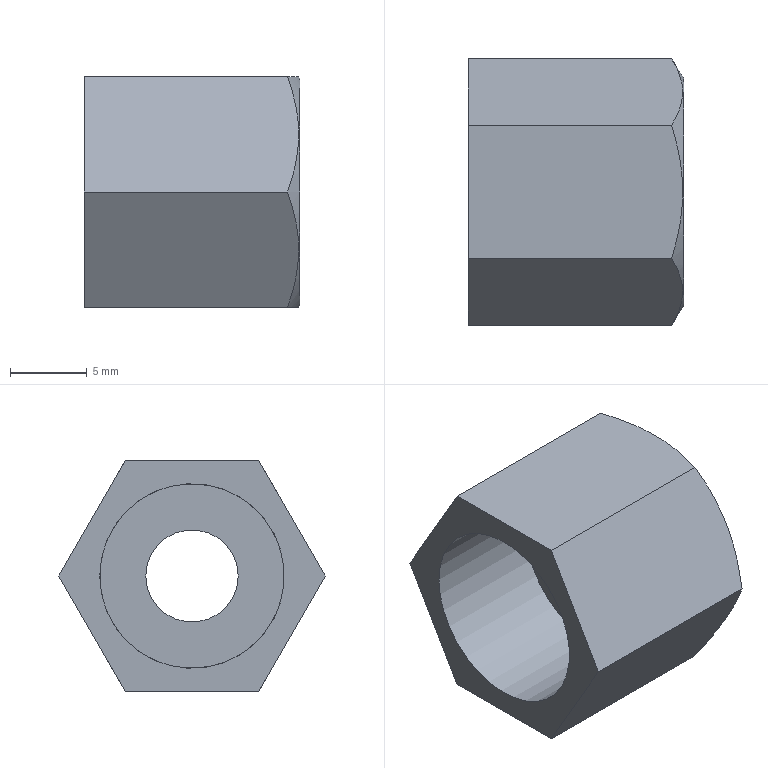Part | STEP file | 1-23.6 | 2 solids | 16 faces | box 14 x 17.321 x 15 mm | volume 1648 mm3 | plane 11 | cylinder 4 | cone 1 | commonest cylinder face diameters 6 x2 12 x2
STEP:
#1=CARTESIAN_POINT('',(0.,0.,0.));
#2=DIRECTION('',(0.,0.,1.));
#3=DIRECTION('',(1.,0.,0.));
#4=AXIS2_PLACEMENT_3D('',#1,#2,#3);
#5=CARTESIAN_POINT('',(0.,-4.33,7.5));
#6=VERTEX_POINT('',#5);
#7=CARTESIAN_POINT('',(0.,4.33,7.5));
#8=VERTEX_POINT('',#7);
#9=CARTESIAN_POINT('',(0.,-4.33,7.5));
#10=DIRECTION('',(0.,1.,0.));
#11=VECTOR('',#10,1.);
#12=LINE('',#9,#11);
#13=CARTESIAN_POINT('',(0.,0.,1.16));
#14=DIRECTION('',(-1.,0.,0.));
#15=DIRECTION('',(0.,0.,1.));
#16=AXIS2_PLACEMENT_3D('',#13,#14,#15);
#17=PLANE('',#16);
#18=CARTESIAN_POINT('',(6.34,-4.33));
#19=DIRECTION('',(0.,1.));
#20=VECTOR('',#19,1.);
#21=LINE('',#18,#20);
#22=(GEOMETRIC_REPRESENTATION_CONTEXT(2)PARAMETRIC_REPRESENTATION_CONTEXT()REPRESENTATION_CONTEXT('',''));
#23=DEFINITIONAL_REPRESENTATION('',(#21),#22);
#24=PCURVE('',#17,#23);
#25=CARTESIAN_POINT('',(7.,0.,7.5));
#26=DIRECTION('',(0.,0.,-1.));
#27=DIRECTION('',(0.,1.,0.));
#28=AXIS2_PLACEMENT_3D('',#25,#26,#27);
#29=PLANE('',#28);
#30=CARTESIAN_POINT('',(-4.33,-7.));
#31=DIRECTION('',(1.,0.));
#32=VECTOR('',#31,1.);
#33=LINE('',#30,#32);
#34=(GEOMETRIC_REPRESENTATION_CONTEXT(2)PARAMETRIC_REPRESENTATION_CONTEXT()REPRESENTATION_CONTEXT('',''));
#35=DEFINITIONAL_REPRESENTATION('',(#33),#34);
#36=PCURVE('',#29,#35);
#37=SURFACE_CURVE('',#12,(#24,#36),.PCURVE_S1.);
#38=EDGE_CURVE('',#6,#8,#37,.T.);
#39=ORIENTED_EDGE('',*,*,#38,.T.);
#40=CARTESIAN_POINT('',(0.,8.66,0.));
#41=VERTEX_POINT('',#40);
#42=CARTESIAN_POINT('',(0.,4.33,7.5));
#43=DIRECTION('',(0.,0.5,-0.866));
#44=VECTOR('',#43,1.);
#45=LINE('',#42,#44);
#46=CARTESIAN_POINT('',(6.34,4.33));
#47=DIRECTION('',(-0.866,0.5));
#48=VECTOR('',#47,1.);
#49=LINE('',#46,#48);
#50=(GEOMETRIC_REPRESENTATION_CONTEXT(2)PARAMETRIC_REPRESENTATION_CONTEXT()REPRESENTATION_CONTEXT('',''));
#51=DEFINITIONAL_REPRESENTATION('',(#49),#50);
#52=PCURVE('',#17,#51);
#53=CARTESIAN_POINT('',(7.,6.495,3.75));
#54=DIRECTION('',(0.,-0.866,-0.5));
#55=DIRECTION('',(0.,0.5,-0.866));
#56=AXIS2_PLACEMENT_3D('',#53,#54,#55);
#57=PLANE('',#56);
#58=CARTESIAN_POINT('',(-4.33,-7.));
#59=DIRECTION('',(1.,0.));
#60=VECTOR('',#59,1.);
#61=LINE('',#58,#60);
#62=(GEOMETRIC_REPRESENTATION_CONTEXT(2)PARAMETRIC_REPRESENTATION_CONTEXT()REPRESENTATION_CONTEXT('',''));
#63=DEFINITIONAL_REPRESENTATION('',(#61),#62);
#64=PCURVE('',#57,#63);
#65=SURFACE_CURVE('',#45,(#52,#64),.PCURVE_S1.);
#66=EDGE_CURVE('',#8,#41,#65,.T.);
#67=ORIENTED_EDGE('',*,*,#66,.T.);
#68=CARTESIAN_POINT('',(0.,4.33,-7.5));
#69=VERTEX_POINT('',#68);
#70=CARTESIAN_POINT('',(0.,8.66,0.));
#71=DIRECTION('',(0.,-0.5,-0.866));
#72=VECTOR('',#71,1.);
#73=LINE('',#70,#72);
#74=CARTESIAN_POINT('',(-1.16,8.66));
#75=DIRECTION('',(-0.866,-0.5));
#76=VECTOR('',#75,1.);
#77=LINE('',#74,#76);
#78=(GEOMETRIC_REPRESENTATION_CONTEXT(2)PARAMETRIC_REPRESENTATION_CONTEXT()REPRESENTATION_CONTEXT('',''));
#79=DEFINITIONAL_REPRESENTATION('',(#77),#78);
#80=PCURVE('',#17,#79);
#81=CARTESIAN_POINT('',(7.,6.495,-3.75));
#82=DIRECTION('',(0.,-0.866,0.5));
#83=DIRECTION('',(0.,-0.5,-0.866));
#84=AXIS2_PLACEMENT_3D('',#81,#82,#83);
#85=PLANE('',#84);
#86=CARTESIAN_POINT('',(-4.33,-7.));
#87=DIRECTION('',(1.,0.));
#88=VECTOR('',#87,1.);
#89=LINE('',#86,#88);
#90=(GEOMETRIC_REPRESENTATION_CONTEXT(2)PARAMETRIC_REPRESENTATION_CONTEXT()REPRESENTATION_CONTEXT('',''));
#91=DEFINITIONAL_REPRESENTATION('',(#89),#90);
#92=PCURVE('',#85,#91);
#93=SURFACE_CURVE('',#73,(#80,#92),.PCURVE_S1.);
#94=EDGE_CURVE('',#41,#69,#93,.T.);
#95=ORIENTED_EDGE('',*,*,#94,.T.);
#96=CARTESIAN_POINT('',(0.,-4.33,-7.5));
#97=VERTEX_POINT('',#96);
#98=CARTESIAN_POINT('',(0.,4.33,-7.5));
#99=DIRECTION('',(0.,-1.,0.));
#100=VECTOR('',#99,1.);
#101=LINE('',#98,#100);
#102=CARTESIAN_POINT('',(-8.66,4.33));
#103=DIRECTION('',(0.,-1.));
#104=VECTOR('',#103,1.);
#105=LINE('',#102,#104);
#106=(GEOMETRIC_REPRESENTATION_CONTEXT(2)PARAMETRIC_REPRESENTATION_CONTEXT()REPRESENTATION_CONTEXT('',''));
#107=DEFINITIONAL_REPRESENTATION('',(#105),#106);
#108=PCURVE('',#17,#107);
#109=CARTESIAN_POINT('',(7.,0.,-7.5));
#110=DIRECTION('',(0.,0.,1.));
#111=DIRECTION('',(0.,-1.,0.));
#112=AXIS2_PLACEMENT_3D('',#109,#110,#111);
#113=PLANE('',#112);
#114=CARTESIAN_POINT('',(-4.33,-7.));
#115=DIRECTION('',(1.,0.));
#116=VECTOR('',#115,1.);
#117=LINE('',#114,#116);
#118=(GEOMETRIC_REPRESENTATION_CONTEXT(2)PARAMETRIC_REPRESENTATION_CONTEXT()REPRESENTATION_CONTEXT('',''));
#119=DEFINITIONAL_REPRESENTATION('',(#117),#118);
#120=PCURVE('',#113,#119);
#121=SURFACE_CURVE('',#101,(#108,#120),.PCURVE_S1.);
#122=EDGE_CURVE('',#69,#97,#121,.T.);
#123=ORIENTED_EDGE('',*,*,#122,.T.);
#124=CARTESIAN_POINT('',(0.,-8.66,0.));
#125=VERTEX_POINT('',#124);
#126=CARTESIAN_POINT('',(0.,-4.33,-7.5));
#127=DIRECTION('',(0.,-0.5,0.866));
#128=VECTOR('',#127,1.);
#129=LINE('',#126,#128);
#130=CARTESIAN_POINT('',(-8.66,-4.33));
#131=DIRECTION('',(0.866,-0.5));
#132=VECTOR('',#131,1.);
#133=LINE('',#130,#132);
#134=(GEOMETRIC_REPRESENTATION_CONTEXT(2)PARAMETRIC_REPRESENTATION_CONTEXT()REPRESENTATION_CONTEXT('',''));
#135=DEFINITIONAL_REPRESENTATION('',(#133),#134);
#136=PCURVE('',#17,#135);
#137=CARTESIAN_POINT('',(7.,-6.495,-3.75));
#138=DIRECTION('',(0.,0.866,0.5));
#139=DIRECTION('',(0.,-0.5,0.866));
#140=AXIS2_PLACEMENT_3D('',#137,#138,#139);
#141=PLANE('',#140);
#142=CARTESIAN_POINT('',(-4.33,-7.));
#143=DIRECTION('',(1.,0.));
#144=VECTOR('',#143,1.);
#145=LINE('',#142,#144);
#146=(GEOMETRIC_REPRESENTATION_CONTEXT(2)PARAMETRIC_REPRESENTATION_CONTEXT()REPRESENTATION_CONTEXT('',''));
#147=DEFINITIONAL_REPRESENTATION('',(#145),#146);
#148=PCURVE('',#141,#147);
#149=SURFACE_CURVE('',#129,(#136,#148),.PCURVE_S1.);
#150=EDGE_CURVE('',#97,#125,#149,.T.);
#151=ORIENTED_EDGE('',*,*,#150,.T.);
#152=CARTESIAN_POINT('',(0.,-8.66,0.));
#153=DIRECTION('',(0.,0.5,0.866));
#154=VECTOR('',#153,1.);
#155=LINE('',#152,#154);
#156=CARTESIAN_POINT('',(-1.16,-8.66));
#157=DIRECTION('',(0.866,0.5));
#158=VECTOR('',#157,1.);
#159=LINE('',#156,#158);
#160=(GEOMETRIC_REPRESENTATION_CONTEXT(2)PARAMETRIC_REPRESENTATION_CONTEXT()REPRESENTATION_CONTEXT('',''));
#161=DEFINITIONAL_REPRESENTATION('',(#159),#160);
#162=PCURVE('',#17,#161);
#163=CARTESIAN_POINT('',(7.,-6.495,3.75));
#164=DIRECTION('',(0.,0.866,-0.5));
#165=DIRECTION('',(0.,0.5,0.866));
#166=AXIS2_PLACEMENT_3D('',#163,#164,#165);
#167=PLANE('',#166);
#168=CARTESIAN_POINT('',(-4.33,-7.));
#169=DIRECTION('',(1.,0.));
#170=VECTOR('',#169,1.);
#171=LINE('',#168,#170);
#172=(GEOMETRIC_REPRESENTATION_CONTEXT(2)PARAMETRIC_REPRESENTATION_CONTEXT()REPRESENTATION_CONTEXT('',''));
#173=DEFINITIONAL_REPRESENTATION('',(#171),#172);
#174=PCURVE('',#167,#173);
#175=SURFACE_CURVE('',#155,(#162,#174),.PCURVE_S1.);
#176=EDGE_CURVE('',#125,#6,#175,.T.);
#177=ORIENTED_EDGE('',*,*,#176,.T.);
#178=EDGE_LOOP('',(#39,#67,#95,#123,#151,#177));
#179=FACE_BOUND('',#178,.T.);
#180=CARTESIAN_POINT('',(0.,6.,0.));
#181=VERTEX_POINT('',#180);
#182=CARTESIAN_POINT('',(0.,0.,0.));
#183=DIRECTION('',(1.,0.,0.));
#184=DIRECTION('',(0.,1.,0.));
#185=AXIS2_PLACEMENT_3D('',#182,#183,#184);
#186=CIRCLE('',#185,6.);
#187=CARTESIAN_POINT('',(-1.16,6.));
#188=CARTESIAN_POINT('',(9.232,6.));
#189=CARTESIAN_POINT('',(4.036,-3.));
#190=CARTESIAN_POINT('',(-1.16,-12.));
#191=CARTESIAN_POINT('',(-6.356,-3.));
#192=CARTESIAN_POINT('',(-11.553,6.));
#193=CARTESIAN_POINT('',(-1.16,6.));
#194=(BOUNDED_CURVE()B_SPLINE_CURVE(2,(#187,#188,#189,#190,#191,#192,#193),.UNSPECIFIED.,.T.,.F.)B_SPLINE_CURVE_WITH_KNOTS((1,2,2,2,2,1),(-2.094,0.,2.094,4.189,6.283,8.378),.UNSPECIFIED.)CURVE()GEOMETRIC_REPRESENTATION_ITEM()RATIONAL_B_SPLINE_CURVE((1.,0.5,1.,0.5,1.,0.5,1.))REPRESENTATION_ITEM(''));
#195=(GEOMETRIC_REPRESENTATION_CONTEXT(2)PARAMETRIC_REPRESENTATION_CONTEXT()REPRESENTATION_CONTEXT('',''));
#196=DEFINITIONAL_REPRESENTATION('',(#194),#195);
#197=PCURVE('',#17,#196);
#198=CARTESIAN_POINT('',(0.,0.,0.));
#199=DIRECTION('',(1.,0.,0.));
#200=DIRECTION('',(0.,1.,0.));
#201=AXIS2_PLACEMENT_3D('',#198,#199,#200);
#202=CYLINDRICAL_SURFACE('',#201,6.);
#203=CARTESIAN_POINT('',(0.,0.));
#204=DIRECTION('',(1.,0.));
#205=VECTOR('',#204,1.);
#206=LINE('',#203,#205);
#207=(GEOMETRIC_REPRESENTATION_CONTEXT(2)PARAMETRIC_REPRESENTATION_CONTEXT()REPRESENTATION_CONTEXT('',''));
#208=DEFINITIONAL_REPRESENTATION('',(#206),#207);
#209=PCURVE('',#202,#208);
#210=SURFACE_CURVE('',#186,(#197,#209),.PCURVE_S1.);
#211=EDGE_CURVE('',#181,#181,#210,.T.);
#212=ORIENTED_EDGE('',*,*,#211,.T.);
#213=EDGE_LOOP('',(#212));
#214=FACE_BOUND('',#213,.T.);
#215=ADVANCED_FACE('',(#179,#214),#17,.T.);
#216=ORIENTED_EDGE('',*,*,#211,.T.);
#217=CARTESIAN_POINT('',(11.,6.,0.));
#218=VERTEX_POINT('',#217);
#219=CARTESIAN_POINT('',(0.,6.,0.));
#220=DIRECTION('',(1.,0.,0.));
#221=VECTOR('',#220,1.);
#222=LINE('',#219,#221);
#223=CARTESIAN_POINT('',(6.283,0.));
#224=DIRECTION('',(0.,1.));
#225=VECTOR('',#224,1.);
#226=LINE('',#223,#225);
#227=(GEOMETRIC_REPRESENTATION_CONTEXT(2)PARAMETRIC_REPRESENTATION_CONTEXT()REPRESENTATION_CONTEXT('',''));
#228=DEFINITIONAL_REPRESENTATION('',(#226),#227);
#229=PCURVE('',#202,#228);
#230=CARTESIAN_POINT('',(0.,0.));
#231=DIRECTION('',(0.,1.));
#232=VECTOR('',#231,1.);
#233=LINE('',#230,#232);
#234=(GEOMETRIC_REPRESENTATION_CONTEXT(2)PARAMETRIC_REPRESENTATION_CONTEXT()REPRESENTATION_CONTEXT('',''));
#235=DEFINITIONAL_REPRESENTATION('',(#233),#234);
#236=PCURVE('',#202,#235);
#237=SEAM_CURVE('',#222,(#229,#236),.PCURVE_S1.);
#238=EDGE_CURVE('',#181,#218,#237,.T.);
#239=ORIENTED_EDGE('',*,*,#238,.T.);
#240=CARTESIAN_POINT('',(11.,0.,0.));
#241=DIRECTION('',(1.,0.,0.));
#242=DIRECTION('',(0.,1.,0.));
#243=AXIS2_PLACEMENT_3D('',#240,#241,#242);
#244=CIRCLE('',#243,6.);
#245=CARTESIAN_POINT('',(0.,11.));
#246=DIRECTION('',(1.,0.));
#247=VECTOR('',#246,1.);
#248=LINE('',#245,#247);
#249=(GEOMETRIC_REPRESENTATION_CONTEXT(2)PARAMETRIC_REPRESENTATION_CONTEXT()REPRESENTATION_CONTEXT('',''));
#250=DEFINITIONAL_REPRESENTATION('',(#248),#249);
#251=PCURVE('',#202,#250);
#252=CARTESIAN_POINT('',(11.,-1.608,0.));
#253=DIRECTION('',(1.,0.,0.));
#254=DIRECTION('',(0.,0.,-1.));
#255=AXIS2_PLACEMENT_3D('',#252,#253,#254);
#256=PLANE('',#255);
#257=CARTESIAN_POINT('',(0.,1.608));
#258=DIRECTION('',(0.,1.));
#259=AXIS2_PLACEMENT_2D('',#257,#258);
#260=CIRCLE('',#259,6.);
#261=(GEOMETRIC_REPRESENTATION_CONTEXT(2)PARAMETRIC_REPRESENTATION_CONTEXT()REPRESENTATION_CONTEXT('',''));
#262=DEFINITIONAL_REPRESENTATION('',(#260),#261);
#263=PCURVE('',#256,#262);
#264=SURFACE_CURVE('',#244,(#251,#263),.PCURVE_S1.);
#265=EDGE_CURVE('',#218,#218,#264,.T.);
#266=ORIENTED_EDGE('',*,*,#265,.F.);
#267=ORIENTED_EDGE('',*,*,#238,.F.);
#268=EDGE_LOOP('',(#216,#239,#266,#267));
#269=FACE_BOUND('',#268,.F.);
#270=ADVANCED_FACE('',(#269),#202,.F.);
#271=ORIENTED_EDGE('',*,*,#38,.T.);
#272=CARTESIAN_POINT('',(13.213,4.33,7.5));
#273=VERTEX_POINT('',#272);
#274=CARTESIAN_POINT('',(0.,4.33,7.5));
#275=DIRECTION('',(1.,0.,0.));
#276=VECTOR('',#275,1.);
#277=LINE('',#274,#276);
#278=CARTESIAN_POINT('',(4.33,-7.));
#279=DIRECTION('',(0.,1.));
#280=VECTOR('',#279,1.);
#281=LINE('',#278,#280);
#282=(GEOMETRIC_REPRESENTATION_CONTEXT(2)PARAMETRIC_REPRESENTATION_CONTEXT()REPRESENTATION_CONTEXT('',''));
#283=DEFINITIONAL_REPRESENTATION('',(#281),#282);
#284=PCURVE('',#29,#283);
#285=CARTESIAN_POINT('',(-4.33,-7.));
#286=DIRECTION('',(0.,1.));
#287=VECTOR('',#286,1.);
#288=LINE('',#285,#287);
#289=(GEOMETRIC_REPRESENTATION_CONTEXT(2)PARAMETRIC_REPRESENTATION_CONTEXT()REPRESENTATION_CONTEXT('',''));
#290=DEFINITIONAL_REPRESENTATION('',(#288),#289);
#291=PCURVE('',#57,#290);
#292=SURFACE_CURVE('',#277,(#284,#291),.PCURVE_S1.);
#293=EDGE_CURVE('',#8,#273,#292,.T.);
#294=ORIENTED_EDGE('',*,*,#293,.T.);
#295=CARTESIAN_POINT('',(13.936,0.,7.5));
#296=VERTEX_POINT('',#295);
#297=CARTESIAN_POINT('',(13.213,4.33,7.5));
#298=CARTESIAN_POINT('',(13.936,2.01,7.5));
#299=CARTESIAN_POINT('',(13.936,0.,7.5));
#300=(BOUNDED_CURVE()B_SPLINE_CURVE(2,(#297,#298,#299),.UNSPECIFIED.,.F.,.F.)B_SPLINE_CURVE_WITH_KNOTS((3,3),(0.,1.),.PIECEWISE_BEZIER_KNOTS.)CURVE()GEOMETRIC_REPRESENTATION_ITEM()RATIONAL_B_SPLINE_CURVE((1.788,1.926,1.926))REPRESENTATION_ITEM(''));
#301=CARTESIAN_POINT('',(4.33,6.213));
#302=CARTESIAN_POINT('',(2.01,6.936));
#303=CARTESIAN_POINT('',(0.,6.936));
#304=(BOUNDED_CURVE()B_SPLINE_CURVE(2,(#301,#302,#303),.UNSPECIFIED.,.F.,.F.)B_SPLINE_CURVE_WITH_KNOTS((3,3),(0.,1.),.PIECEWISE_BEZIER_KNOTS.)CURVE()GEOMETRIC_REPRESENTATION_ITEM()RATIONAL_B_SPLINE_CURVE((1.788,1.926,1.926))REPRESENTATION_ITEM(''));
#305=(GEOMETRIC_REPRESENTATION_CONTEXT(2)PARAMETRIC_REPRESENTATION_CONTEXT()REPRESENTATION_CONTEXT('',''));
#306=DEFINITIONAL_REPRESENTATION('',(#304),#305);
#307=PCURVE('',#29,#306);
#308=CARTESIAN_POINT('',(14.,0.,0.));
#309=DIRECTION('',(-1.,0.,0.));
#310=DIRECTION('',(0.,0.,1.));
#311=AXIS2_PLACEMENT_3D('',#308,#309,#310);
#312=CONICAL_SURFACE('',#311,7.397,1.014);
#313=CARTESIAN_POINT('',(0.5236,0.7867));
#314=CARTESIAN_POINT('',(0.516,0.7631));
#315=CARTESIAN_POINT('',(0.5008,0.7174));
#316=CARTESIAN_POINT('',(0.4779,0.6528));
#317=CARTESIAN_POINT('',(0.4548,0.5921));
#318=CARTESIAN_POINT('',(0.4317,0.5352));
#319=CARTESIAN_POINT('',(0.4084,0.482));
#320=CARTESIAN_POINT('',(0.3849,0.4324));
#321=CARTESIAN_POINT('',(0.3614,0.3862));
#322=CARTESIAN_POINT('',(0.3378,0.3434));
#323=CARTESIAN_POINT('',(0.3141,0.3039));
#324=CARTESIAN_POINT('',(0.2903,0.2677));
#325=CARTESIAN_POINT('',(0.2664,0.2345));
#326=CARTESIAN_POINT('',(0.2424,0.2044));
#327=CARTESIAN_POINT('',(0.2184,0.1774));
#328=CARTESIAN_POINT('',(0.1943,0.1534));
#329=CARTESIAN_POINT('',(0.1701,0.1322));
#330=CARTESIAN_POINT('',(0.1459,0.114));
#331=CARTESIAN_POINT('',(0.1217,0.09862));
#332=CARTESIAN_POINT('',(0.09736,0.08608));
#333=CARTESIAN_POINT('',(0.07305,0.07635));
#334=CARTESIAN_POINT('',(0.04871,0.06941));
#335=CARTESIAN_POINT('',(0.02436,0.06525));
#336=CARTESIAN_POINT('',(0.00812,0.06433));
#337=CARTESIAN_POINT('',(0.,0.06433));
#338=B_SPLINE_CURVE_WITH_KNOTS('',3,(#313,#314,#315,#316,#317,#318,#319,#320,#321,#322,#323,#324,#325,#326,#327,#328,#329,#330,#331,#332,#333,#334,#335,#336,#337),.UNSPECIFIED.,.F.,.F.,(4,1,1,1,1,1,1,1,1,1,1,1,1,1,1,1,1,1,1,1,1,1,4),(0.,0.04545,0.09091,0.1364,0.1818,0.2273,0.2727,0.3182,0.3636,0.4091,0.4545,0.5,0.5455,0.5909,0.6364,0.6818,0.7273,0.7727,0.8182,0.8636,0.9091,0.9545,1.),.QUASI_UNIFORM_KNOTS.);
#339=(GEOMETRIC_REPRESENTATION_CONTEXT(2)PARAMETRIC_REPRESENTATION_CONTEXT()REPRESENTATION_CONTEXT('',''));
#340=DEFINITIONAL_REPRESENTATION('',(#338),#339);
#341=PCURVE('',#312,#340);
#342=SURFACE_CURVE('',#300,(#307,#341),.PCURVE_S1.);
#343=EDGE_CURVE('',#273,#296,#342,.T.);
#344=ORIENTED_EDGE('',*,*,#343,.T.);
#345=CARTESIAN_POINT('',(13.213,-4.33,7.5));
#346=VERTEX_POINT('',#345);
#347=CARTESIAN_POINT('',(13.936,0.,7.5));
#348=CARTESIAN_POINT('',(13.936,-2.01,7.5));
#349=CARTESIAN_POINT('',(13.213,-4.33,7.5));
#350=(BOUNDED_CURVE()B_SPLINE_CURVE(2,(#347,#348,#349),.UNSPECIFIED.,.F.,.F.)B_SPLINE_CURVE_WITH_KNOTS((3,3),(0.,1.),.PIECEWISE_BEZIER_KNOTS.)CURVE()GEOMETRIC_REPRESENTATION_ITEM()RATIONAL_B_SPLINE_CURVE((1.926,1.926,1.788))REPRESENTATION_ITEM(''));
#351=CARTESIAN_POINT('',(0.,6.936));
#352=CARTESIAN_POINT('',(-2.01,6.936));
#353=CARTESIAN_POINT('',(-4.33,6.213));
#354=(BOUNDED_CURVE()B_SPLINE_CURVE(2,(#351,#352,#353),.UNSPECIFIED.,.F.,.F.)B_SPLINE_CURVE_WITH_KNOTS((3,3),(0.,1.),.PIECEWISE_BEZIER_KNOTS.)CURVE()GEOMETRIC_REPRESENTATION_ITEM()RATIONAL_B_SPLINE_CURVE((1.926,1.926,1.788))REPRESENTATION_ITEM(''));
#355=(GEOMETRIC_REPRESENTATION_CONTEXT(2)PARAMETRIC_REPRESENTATION_CONTEXT()REPRESENTATION_CONTEXT('',''));
#356=DEFINITIONAL_REPRESENTATION('',(#354),#355);
#357=PCURVE('',#29,#356);
#358=CARTESIAN_POINT('',(6.283,0.06433));
#359=CARTESIAN_POINT('',(6.275,0.06433));
#360=CARTESIAN_POINT('',(6.259,0.06525));
#361=CARTESIAN_POINT('',(6.234,0.06941));
#362=CARTESIAN_POINT('',(6.21,0.07635));
#363=CARTESIAN_POINT('',(6.186,0.08608));
#364=CARTESIAN_POINT('',(6.162,0.09862));
#365=CARTESIAN_POINT('',(6.137,0.114));
#366=CARTESIAN_POINT('',(6.113,0.1322));
#367=CARTESIAN_POINT('',(6.089,0.1534));
#368=CARTESIAN_POINT('',(6.065,0.1774));
#369=CARTESIAN_POINT('',(6.041,0.2044));
#370=CARTESIAN_POINT('',(6.017,0.2345));
#371=CARTESIAN_POINT('',(5.993,0.2677));
#372=CARTESIAN_POINT('',(5.969,0.3039));
#373=CARTESIAN_POINT('',(5.945,0.3434));
#374=CARTESIAN_POINT('',(5.922,0.3862));
#375=CARTESIAN_POINT('',(5.898,0.4324));
#376=CARTESIAN_POINT('',(5.875,0.482));
#377=CARTESIAN_POINT('',(5.852,0.5352));
#378=CARTESIAN_POINT('',(5.828,0.5921));
#379=CARTESIAN_POINT('',(5.805,0.6528));
#380=CARTESIAN_POINT('',(5.782,0.7174));
#381=CARTESIAN_POINT('',(5.767,0.7631));
#382=CARTESIAN_POINT('',(5.76,0.7867));
#383=B_SPLINE_CURVE_WITH_KNOTS('',3,(#358,#359,#360,#361,#362,#363,#364,#365,#366,#367,#368,#369,#370,#371,#372,#373,#374,#375,#376,#377,#378,#379,#380,#381,#382),.UNSPECIFIED.,.F.,.F.,(4,1,1,1,1,1,1,1,1,1,1,1,1,1,1,1,1,1,1,1,1,1,4),(0.,0.04545,0.09091,0.1364,0.1818,0.2273,0.2727,0.3182,0.3636,0.4091,0.4545,0.5,0.5455,0.5909,0.6364,0.6818,0.7273,0.7727,0.8182,0.8636,0.9091,0.9545,1.),.QUASI_UNIFORM_KNOTS.);
#384=(GEOMETRIC_REPRESENTATION_CONTEXT(2)PARAMETRIC_REPRESENTATION_CONTEXT()REPRESENTATION_CONTEXT('',''));
#385=DEFINITIONAL_REPRESENTATION('',(#383),#384);
#386=PCURVE('',#312,#385);
#387=SURFACE_CURVE('',#350,(#357,#386),.PCURVE_S1.);
#388=EDGE_CURVE('',#296,#346,#387,.T.);
#389=ORIENTED_EDGE('',*,*,#388,.T.);
#390=CARTESIAN_POINT('',(0.,-4.33,7.5));
#391=DIRECTION('',(1.,0.,0.));
#392=VECTOR('',#391,1.);
#393=LINE('',#390,#392);
#394=CARTESIAN_POINT('',(-4.33,-7.));
#395=DIRECTION('',(0.,1.));
#396=VECTOR('',#395,1.);
#397=LINE('',#394,#396);
#398=(GEOMETRIC_REPRESENTATION_CONTEXT(2)PARAMETRIC_REPRESENTATION_CONTEXT()REPRESENTATION_CONTEXT('',''));
#399=DEFINITIONAL_REPRESENTATION('',(#397),#398);
#400=PCURVE('',#29,#399);
#401=CARTESIAN_POINT('',(4.33,-7.));
#402=DIRECTION('',(0.,1.));
#403=VECTOR('',#402,1.);
#404=LINE('',#401,#403);
#405=(GEOMETRIC_REPRESENTATION_CONTEXT(2)PARAMETRIC_REPRESENTATION_CONTEXT()REPRESENTATION_CONTEXT('',''));
#406=DEFINITIONAL_REPRESENTATION('',(#404),#405);
#407=PCURVE('',#167,#406);
#408=SURFACE_CURVE('',#393,(#400,#407),.PCURVE_S1.);
#409=EDGE_CURVE('',#6,#346,#408,.T.);
#410=ORIENTED_EDGE('',*,*,#409,.F.);
#411=EDGE_LOOP('',(#271,#294,#344,#389,#410));
#412=FACE_BOUND('',#411,.F.);
#413=ADVANCED_FACE('',(#412),#29,.F.);
#414=ORIENTED_EDGE('',*,*,#66,.T.);
#415=CARTESIAN_POINT('',(13.213,8.66,0.));
#416=VERTEX_POINT('',#415);
#417=CARTESIAN_POINT('',(0.,8.66,0.));
#418=DIRECTION('',(1.,0.,0.));
#419=VECTOR('',#418,1.);
#420=LINE('',#417,#419);
#421=CARTESIAN_POINT('',(4.33,-7.));
#422=DIRECTION('',(0.,1.));
#423=VECTOR('',#422,1.);
#424=LINE('',#421,#423);
#425=(GEOMETRIC_REPRESENTATION_CONTEXT(2)PARAMETRIC_REPRESENTATION_CONTEXT()REPRESENTATION_CONTEXT('',''));
#426=DEFINITIONAL_REPRESENTATION('',(#424),#425);
#427=PCURVE('',#57,#426);
#428=CARTESIAN_POINT('',(-4.33,-7.));
#429=DIRECTION('',(0.,1.));
#430=VECTOR('',#429,1.);
#431=LINE('',#428,#430);
#432=(GEOMETRIC_REPRESENTATION_CONTEXT(2)PARAMETRIC_REPRESENTATION_CONTEXT()REPRESENTATION_CONTEXT('',''));
#433=DEFINITIONAL_REPRESENTATION('',(#431),#432);
#434=PCURVE('',#85,#433);
#435=SURFACE_CURVE('',#420,(#427,#434),.PCURVE_S1.);
#436=EDGE_CURVE('',#41,#416,#435,.T.);
#437=ORIENTED_EDGE('',*,*,#436,.T.);
#438=CARTESIAN_POINT('',(13.213,8.66,0.));
#439=CARTESIAN_POINT('',(14.561,6.495,3.75));
#440=CARTESIAN_POINT('',(13.213,4.33,7.5));
#441=(BOUNDED_CURVE()B_SPLINE_CURVE(2,(#438,#439,#440),.UNSPECIFIED.,.F.,.F.)B_SPLINE_CURVE_WITH_KNOTS((3,3),(0.,1.),.PIECEWISE_BEZIER_KNOTS.)CURVE()GEOMETRIC_REPRESENTATION_ITEM()RATIONAL_B_SPLINE_CURVE((1.788,2.064,1.788))REPRESENTATION_ITEM(''));
#442=CARTESIAN_POINT('',(4.33,6.213));
#443=CARTESIAN_POINT('',(0.,7.561));
#444=CARTESIAN_POINT('',(-4.33,6.213));
#445=(BOUNDED_CURVE()B_SPLINE_CURVE(2,(#442,#443,#444),.UNSPECIFIED.,.F.,.F.)B_SPLINE_CURVE_WITH_KNOTS((3,3),(0.,1.),.PIECEWISE_BEZIER_KNOTS.)CURVE()GEOMETRIC_REPRESENTATION_ITEM()RATIONAL_B_SPLINE_CURVE((1.788,2.064,1.788))REPRESENTATION_ITEM(''));
#446=(GEOMETRIC_REPRESENTATION_CONTEXT(2)PARAMETRIC_REPRESENTATION_CONTEXT()REPRESENTATION_CONTEXT('',''));
#447=DEFINITIONAL_REPRESENTATION('',(#445),#446);
#448=PCURVE('',#57,#447);
#449=CARTESIAN_POINT('',(1.571,0.7867));
#450=CARTESIAN_POINT('',(1.556,0.7396));
#451=CARTESIAN_POINT('',(1.525,0.6508));
#452=CARTESIAN_POINT('',(1.479,0.5334));
#453=CARTESIAN_POINT('',(1.432,0.4307));
#454=CARTESIAN_POINT('',(1.385,0.3418));
#455=CARTESIAN_POINT('',(1.338,0.2661));
#456=CARTESIAN_POINT('',(1.29,0.2029));
#457=CARTESIAN_POINT('',(1.241,0.1519));
#458=CARTESIAN_POINT('',(1.193,0.1126));
#459=CARTESIAN_POINT('',(1.145,0.08467));
#460=CARTESIAN_POINT('',(1.096,0.06802));
#461=CARTESIAN_POINT('',(1.047,0.06248));
#462=CARTESIAN_POINT('',(0.9985,0.06802));
#463=CARTESIAN_POINT('',(0.9498,0.08467));
#464=CARTESIAN_POINT('',(0.9013,0.1126));
#465=CARTESIAN_POINT('',(0.8529,0.1519));
#466=CARTESIAN_POINT('',(0.8048,0.2029));
#467=CARTESIAN_POINT('',(0.7569,0.2661));
#468=CARTESIAN_POINT('',(0.7094,0.3418));
#469=CARTESIAN_POINT('',(0.6622,0.4307));
#470=CARTESIAN_POINT('',(0.6155,0.5334));
#471=CARTESIAN_POINT('',(0.5692,0.6508));
#472=CARTESIAN_POINT('',(0.5388,0.7396));
#473=CARTESIAN_POINT('',(0.5236,0.7867));
#474=B_SPLINE_CURVE_WITH_KNOTS('',3,(#449,#450,#451,#452,#453,#454,#455,#456,#457,#458,#459,#460,#461,#462,#463,#464,#465,#466,#467,#468,#469,#470,#471,#472,#473),.UNSPECIFIED.,.F.,.F.,(4,1,1,1,1,1,1,1,1,1,1,1,1,1,1,1,1,1,1,1,1,1,4),(0.,0.04545,0.09091,0.1364,0.1818,0.2273,0.2727,0.3182,0.3636,0.4091,0.4545,0.5,0.5455,0.5909,0.6364,0.6818,0.7273,0.7727,0.8182,0.8636,0.9091,0.9545,1.),.QUASI_UNIFORM_KNOTS.);
#475=(GEOMETRIC_REPRESENTATION_CONTEXT(2)PARAMETRIC_REPRESENTATION_CONTEXT()REPRESENTATION_CONTEXT('',''));
#476=DEFINITIONAL_REPRESENTATION('',(#474),#475);
#477=PCURVE('',#312,#476);
#478=SURFACE_CURVE('',#441,(#448,#477),.PCURVE_S1.);
#479=EDGE_CURVE('',#416,#273,#478,.T.);
#480=ORIENTED_EDGE('',*,*,#479,.T.);
#481=ORIENTED_EDGE('',*,*,#293,.F.);
#482=EDGE_LOOP('',(#414,#437,#480,#481));
#483=FACE_BOUND('',#482,.F.);
#484=ADVANCED_FACE('',(#483),#57,.F.);
#485=ORIENTED_EDGE('',*,*,#94,.T.);
#486=CARTESIAN_POINT('',(13.213,4.33,-7.5));
#487=VERTEX_POINT('',#486);
#488=CARTESIAN_POINT('',(0.,4.33,-7.5));
#489=DIRECTION('',(1.,0.,0.));
#490=VECTOR('',#489,1.);
#491=LINE('',#488,#490);
#492=CARTESIAN_POINT('',(4.33,-7.));
#493=DIRECTION('',(0.,1.));
#494=VECTOR('',#493,1.);
#495=LINE('',#492,#494);
#496=(GEOMETRIC_REPRESENTATION_CONTEXT(2)PARAMETRIC_REPRESENTATION_CONTEXT()REPRESENTATION_CONTEXT('',''));
#497=DEFINITIONAL_REPRESENTATION('',(#495),#496);
#498=PCURVE('',#85,#497);
#499=CARTESIAN_POINT('',(-4.33,-7.));
#500=DIRECTION('',(0.,1.));
#501=VECTOR('',#500,1.);
#502=LINE('',#499,#501);
#503=(GEOMETRIC_REPRESENTATION_CONTEXT(2)PARAMETRIC_REPRESENTATION_CONTEXT()REPRESENTATION_CONTEXT('',''));
#504=DEFINITIONAL_REPRESENTATION('',(#502),#503);
#505=PCURVE('',#113,#504);
#506=SURFACE_CURVE('',#491,(#498,#505),.PCURVE_S1.);
#507=EDGE_CURVE('',#69,#487,#506,.T.);
#508=ORIENTED_EDGE('',*,*,#507,.T.);
#509=CARTESIAN_POINT('',(13.213,4.33,-7.5));
#510=CARTESIAN_POINT('',(14.561,6.495,-3.75));
#511=CARTESIAN_POINT('',(13.213,8.66,0.));
#512=(BOUNDED_CURVE()B_SPLINE_CURVE(2,(#509,#510,#511),.UNSPECIFIED.,.F.,.F.)B_SPLINE_CURVE_WITH_KNOTS((3,3),(0.,1.),.PIECEWISE_BEZIER_KNOTS.)CURVE()GEOMETRIC_REPRESENTATION_ITEM()RATIONAL_B_SPLINE_CURVE((1.788,2.064,1.788))REPRESENTATION_ITEM(''));
#513=CARTESIAN_POINT('',(4.33,6.213));
#514=CARTESIAN_POINT('',(0.,7.561));
#515=CARTESIAN_POINT('',(-4.33,6.213));
#516=(BOUNDED_CURVE()B_SPLINE_CURVE(2,(#513,#514,#515),.UNSPECIFIED.,.F.,.F.)B_SPLINE_CURVE_WITH_KNOTS((3,3),(0.,1.),.PIECEWISE_BEZIER_KNOTS.)CURVE()GEOMETRIC_REPRESENTATION_ITEM()RATIONAL_B_SPLINE_CURVE((1.788,2.064,1.788))REPRESENTATION_ITEM(''));
#517=(GEOMETRIC_REPRESENTATION_CONTEXT(2)PARAMETRIC_REPRESENTATION_CONTEXT()REPRESENTATION_CONTEXT('',''));
#518=DEFINITIONAL_REPRESENTATION('',(#516),#517);
#519=PCURVE('',#85,#518);
#520=CARTESIAN_POINT('',(2.618,0.7867));
#521=CARTESIAN_POINT('',(2.603,0.7396));
#522=CARTESIAN_POINT('',(2.572,0.6508));
#523=CARTESIAN_POINT('',(2.526,0.5334));
#524=CARTESIAN_POINT('',(2.479,0.4307));
#525=CARTESIAN_POINT('',(2.432,0.3418));
#526=CARTESIAN_POINT('',(2.385,0.2661));
#527=CARTESIAN_POINT('',(2.337,0.2029));
#528=CARTESIAN_POINT('',(2.289,0.1519));
#529=CARTESIAN_POINT('',(2.24,0.1126));
#530=CARTESIAN_POINT('',(2.192,0.08467));
#531=CARTESIAN_POINT('',(2.143,0.06802));
#532=CARTESIAN_POINT('',(2.094,0.06248));
#533=CARTESIAN_POINT('',(2.046,0.06802));
#534=CARTESIAN_POINT('',(1.997,0.08467));
#535=CARTESIAN_POINT('',(1.948,0.1126));
#536=CARTESIAN_POINT('',(1.9,0.1519));
#537=CARTESIAN_POINT('',(1.852,0.2029));
#538=CARTESIAN_POINT('',(1.804,0.2661));
#539=CARTESIAN_POINT('',(1.757,0.3418));
#540=CARTESIAN_POINT('',(1.709,0.4307));
#541=CARTESIAN_POINT('',(1.663,0.5334));
#542=CARTESIAN_POINT('',(1.616,0.6508));
#543=CARTESIAN_POINT('',(1.586,0.7396));
#544=CARTESIAN_POINT('',(1.571,0.7867));
#545=B_SPLINE_CURVE_WITH_KNOTS('',3,(#520,#521,#522,#523,#524,#525,#526,#527,#528,#529,#530,#531,#532,#533,#534,#535,#536,#537,#538,#539,#540,#541,#542,#543,#544),.UNSPECIFIED.,.F.,.F.,(4,1,1,1,1,1,1,1,1,1,1,1,1,1,1,1,1,1,1,1,1,1,4),(0.,0.04545,0.09091,0.1364,0.1818,0.2273,0.2727,0.3182,0.3636,0.4091,0.4545,0.5,0.5455,0.5909,0.6364,0.6818,0.7273,0.7727,0.8182,0.8636,0.9091,0.9545,1.),.QUASI_UNIFORM_KNOTS.);
#546=(GEOMETRIC_REPRESENTATION_CONTEXT(2)PARAMETRIC_REPRESENTATION_CONTEXT()REPRESENTATION_CONTEXT('',''));
#547=DEFINITIONAL_REPRESENTATION('',(#545),#546);
#548=PCURVE('',#312,#547);
#549=SURFACE_CURVE('',#512,(#519,#548),.PCURVE_S1.);
#550=EDGE_CURVE('',#487,#416,#549,.T.);
#551=ORIENTED_EDGE('',*,*,#550,.T.);
#552=ORIENTED_EDGE('',*,*,#436,.F.);
#553=EDGE_LOOP('',(#485,#508,#551,#552));
#554=FACE_BOUND('',#553,.F.);
#555=ADVANCED_FACE('',(#554),#85,.F.);
#556=ORIENTED_EDGE('',*,*,#122,.T.);
#557=CARTESIAN_POINT('',(13.213,-4.33,-7.5));
#558=VERTEX_POINT('',#557);
#559=CARTESIAN_POINT('',(0.,-4.33,-7.5));
#560=DIRECTION('',(1.,0.,0.));
#561=VECTOR('',#560,1.);
#562=LINE('',#559,#561);
#563=CARTESIAN_POINT('',(4.33,-7.));
#564=DIRECTION('',(0.,1.));
#565=VECTOR('',#564,1.);
#566=LINE('',#563,#565);
#567=(GEOMETRIC_REPRESENTATION_CONTEXT(2)PARAMETRIC_REPRESENTATION_CONTEXT()REPRESENTATION_CONTEXT('',''));
#568=DEFINITIONAL_REPRESENTATION('',(#566),#567);
#569=PCURVE('',#113,#568);
#570=CARTESIAN_POINT('',(-4.33,-7.));
#571=DIRECTION('',(0.,1.));
#572=VECTOR('',#571,1.);
#573=LINE('',#570,#572);
#574=(GEOMETRIC_REPRESENTATION_CONTEXT(2)PARAMETRIC_REPRESENTATION_CONTEXT()REPRESENTATION_CONTEXT('',''));
#575=DEFINITIONAL_REPRESENTATION('',(#573),#574);
#576=PCURVE('',#141,#575);
#577=SURFACE_CURVE('',#562,(#569,#576),.PCURVE_S1.);
#578=EDGE_CURVE('',#97,#558,#577,.T.);
#579=ORIENTED_EDGE('',*,*,#578,.T.);
#580=CARTESIAN_POINT('',(13.213,-4.33,-7.5));
#581=CARTESIAN_POINT('',(14.561,0.,-7.5));
#582=CARTESIAN_POINT('',(13.213,4.33,-7.5));
#583=(BOUNDED_CURVE()B_SPLINE_CURVE(2,(#580,#581,#582),.UNSPECIFIED.,.F.,.F.)B_SPLINE_CURVE_WITH_KNOTS((3,3),(0.,1.),.PIECEWISE_BEZIER_KNOTS.)CURVE()GEOMETRIC_REPRESENTATION_ITEM()RATIONAL_B_SPLINE_CURVE((1.788,2.064,1.788))REPRESENTATION_ITEM(''));
#584=CARTESIAN_POINT('',(4.33,6.213));
#585=CARTESIAN_POINT('',(0.,7.561));
#586=CARTESIAN_POINT('',(-4.33,6.213));
#587=(BOUNDED_CURVE()B_SPLINE_CURVE(2,(#584,#585,#586),.UNSPECIFIED.,.F.,.F.)B_SPLINE_CURVE_WITH_KNOTS((3,3),(0.,1.),.PIECEWISE_BEZIER_KNOTS.)CURVE()GEOMETRIC_REPRESENTATION_ITEM()RATIONAL_B_SPLINE_CURVE((1.788,2.064,1.788))REPRESENTATION_ITEM(''));
#588=(GEOMETRIC_REPRESENTATION_CONTEXT(2)PARAMETRIC_REPRESENTATION_CONTEXT()REPRESENTATION_CONTEXT('',''));
#589=DEFINITIONAL_REPRESENTATION('',(#587),#588);
#590=PCURVE('',#113,#589);
#591=CARTESIAN_POINT('',(3.665,0.7867));
#592=CARTESIAN_POINT('',(3.65,0.7396));
#593=CARTESIAN_POINT('',(3.62,0.6508));
#594=CARTESIAN_POINT('',(3.573,0.5334));
#595=CARTESIAN_POINT('',(3.527,0.4307));
#596=CARTESIAN_POINT('',(3.479,0.3418));
#597=CARTESIAN_POINT('',(3.432,0.2661));
#598=CARTESIAN_POINT('',(3.384,0.2029));
#599=CARTESIAN_POINT('',(3.336,0.1519));
#600=CARTESIAN_POINT('',(3.288,0.1126));
#601=CARTESIAN_POINT('',(3.239,0.08467));
#602=CARTESIAN_POINT('',(3.19,0.06802));
#603=CARTESIAN_POINT('',(3.142,0.06248));
#604=CARTESIAN_POINT('',(3.093,0.06802));
#605=CARTESIAN_POINT('',(3.044,0.08467));
#606=CARTESIAN_POINT('',(2.996,0.1126));
#607=CARTESIAN_POINT('',(2.947,0.1519));
#608=CARTESIAN_POINT('',(2.899,0.2029));
#609=CARTESIAN_POINT('',(2.851,0.2661));
#610=CARTESIAN_POINT('',(2.804,0.3418));
#611=CARTESIAN_POINT('',(2.757,0.4307));
#612=CARTESIAN_POINT('',(2.71,0.5334));
#613=CARTESIAN_POINT('',(2.664,0.6508));
#614=CARTESIAN_POINT('',(2.633,0.7396));
#615=CARTESIAN_POINT('',(2.618,0.7867));
#616=B_SPLINE_CURVE_WITH_KNOTS('',3,(#591,#592,#593,#594,#595,#596,#597,#598,#599,#600,#601,#602,#603,#604,#605,#606,#607,#608,#609,#610,#611,#612,#613,#614,#615),.UNSPECIFIED.,.F.,.F.,(4,1,1,1,1,1,1,1,1,1,1,1,1,1,1,1,1,1,1,1,1,1,4),(0.,0.04545,0.09091,0.1364,0.1818,0.2273,0.2727,0.3182,0.3636,0.4091,0.4545,0.5,0.5455,0.5909,0.6364,0.6818,0.7273,0.7727,0.8182,0.8636,0.9091,0.9545,1.),.QUASI_UNIFORM_KNOTS.);
#617=(GEOMETRIC_REPRESENTATION_CONTEXT(2)PARAMETRIC_REPRESENTATION_CONTEXT()REPRESENTATION_CONTEXT('',''));
#618=DEFINITIONAL_REPRESENTATION('',(#616),#617);
#619=PCURVE('',#312,#618);
#620=SURFACE_CURVE('',#583,(#590,#619),.PCURVE_S1.);
#621=EDGE_CURVE('',#558,#487,#620,.T.);
#622=ORIENTED_EDGE('',*,*,#621,.T.);
#623=ORIENTED_EDGE('',*,*,#507,.F.);
#624=EDGE_LOOP('',(#556,#579,#622,#623));
#625=FACE_BOUND('',#624,.F.);
#626=ADVANCED_FACE('',(#625),#113,.F.);
#627=ORIENTED_EDGE('',*,*,#150,.T.);
#628=CARTESIAN_POINT('',(13.213,-8.66,0.));
#629=VERTEX_POINT('',#628);
#630=CARTESIAN_POINT('',(0.,-8.66,0.));
#631=DIRECTION('',(1.,0.,0.));
#632=VECTOR('',#631,1.);
#633=LINE('',#630,#632);
#634=CARTESIAN_POINT('',(4.33,-7.));
#635=DIRECTION('',(0.,1.));
#636=VECTOR('',#635,1.);
#637=LINE('',#634,#636);
#638=(GEOMETRIC_REPRESENTATION_CONTEXT(2)PARAMETRIC_REPRESENTATION_CONTEXT()REPRESENTATION_CONTEXT('',''));
#639=DEFINITIONAL_REPRESENTATION('',(#637),#638);
#640=PCURVE('',#141,#639);
#641=CARTESIAN_POINT('',(-4.33,-7.));
#642=DIRECTION('',(0.,1.));
#643=VECTOR('',#642,1.);
#644=LINE('',#641,#643);
#645=(GEOMETRIC_REPRESENTATION_CONTEXT(2)PARAMETRIC_REPRESENTATION_CONTEXT()REPRESENTATION_CONTEXT('',''));
#646=DEFINITIONAL_REPRESENTATION('',(#644),#645);
#647=PCURVE('',#167,#646);
#648=SURFACE_CURVE('',#633,(#640,#647),.PCURVE_S1.);
#649=EDGE_CURVE('',#125,#629,#648,.T.);
#650=ORIENTED_EDGE('',*,*,#649,.T.);
#651=CARTESIAN_POINT('',(13.213,-8.66,0.));
#652=CARTESIAN_POINT('',(14.561,-6.495,-3.75));
#653=CARTESIAN_POINT('',(13.213,-4.33,-7.5));
#654=(BOUNDED_CURVE()B_SPLINE_CURVE(2,(#651,#652,#653),.UNSPECIFIED.,.F.,.F.)B_SPLINE_CURVE_WITH_KNOTS((3,3),(0.,1.),.PIECEWISE_BEZIER_KNOTS.)CURVE()GEOMETRIC_REPRESENTATION_ITEM()RATIONAL_B_SPLINE_CURVE((1.788,2.064,1.788))REPRESENTATION_ITEM(''));
#655=CARTESIAN_POINT('',(4.33,6.213));
#656=CARTESIAN_POINT('',(0.,7.561));
#657=CARTESIAN_POINT('',(-4.33,6.213));
#658=(BOUNDED_CURVE()B_SPLINE_CURVE(2,(#655,#656,#657),.UNSPECIFIED.,.F.,.F.)B_SPLINE_CURVE_WITH_KNOTS((3,3),(0.,1.),.PIECEWISE_BEZIER_KNOTS.)CURVE()GEOMETRIC_REPRESENTATION_ITEM()RATIONAL_B_SPLINE_CURVE((1.788,2.064,1.788))REPRESENTATION_ITEM(''));
#659=(GEOMETRIC_REPRESENTATION_CONTEXT(2)PARAMETRIC_REPRESENTATION_CONTEXT()REPRESENTATION_CONTEXT('',''));
#660=DEFINITIONAL_REPRESENTATION('',(#658),#659);
#661=PCURVE('',#141,#660);
#662=CARTESIAN_POINT('',(4.712,0.7867));
#663=CARTESIAN_POINT('',(4.697,0.7396));
#664=CARTESIAN_POINT('',(4.667,0.6508));
#665=CARTESIAN_POINT('',(4.621,0.5334));
#666=CARTESIAN_POINT('',(4.574,0.4307));
#667=CARTESIAN_POINT('',(4.527,0.3418));
#668=CARTESIAN_POINT('',(4.479,0.2661));
#669=CARTESIAN_POINT('',(4.431,0.2029));
#670=CARTESIAN_POINT('',(4.383,0.1519));
#671=CARTESIAN_POINT('',(4.335,0.1126));
#672=CARTESIAN_POINT('',(4.286,0.08467));
#673=CARTESIAN_POINT('',(4.238,0.06802));
#674=CARTESIAN_POINT('',(4.189,0.06248));
#675=CARTESIAN_POINT('',(4.14,0.06802));
#676=CARTESIAN_POINT('',(4.091,0.08467));
#677=CARTESIAN_POINT('',(4.043,0.1126));
#678=CARTESIAN_POINT('',(3.994,0.1519));
#679=CARTESIAN_POINT('',(3.946,0.2029));
#680=CARTESIAN_POINT('',(3.898,0.2661));
#681=CARTESIAN_POINT('',(3.851,0.3418));
#682=CARTESIAN_POINT('',(3.804,0.4307));
#683=CARTESIAN_POINT('',(3.757,0.5334));
#684=CARTESIAN_POINT('',(3.711,0.6508));
#685=CARTESIAN_POINT('',(3.68,0.7396));
#686=CARTESIAN_POINT('',(3.665,0.7867));
#687=B_SPLINE_CURVE_WITH_KNOTS('',3,(#662,#663,#664,#665,#666,#667,#668,#669,#670,#671,#672,#673,#674,#675,#676,#677,#678,#679,#680,#681,#682,#683,#684,#685,#686),.UNSPECIFIED.,.F.,.F.,(4,1,1,1,1,1,1,1,1,1,1,1,1,1,1,1,1,1,1,1,1,1,4),(0.,0.04545,0.09091,0.1364,0.1818,0.2273,0.2727,0.3182,0.3636,0.4091,0.4545,0.5,0.5455,0.5909,0.6364,0.6818,0.7273,0.7727,0.8182,0.8636,0.9091,0.9545,1.),.QUASI_UNIFORM_KNOTS.);
#688=(GEOMETRIC_REPRESENTATION_CONTEXT(2)PARAMETRIC_REPRESENTATION_CONTEXT()REPRESENTATION_CONTEXT('',''));
#689=DEFINITIONAL_REPRESENTATION('',(#687),#688);
#690=PCURVE('',#312,#689);
#691=SURFACE_CURVE('',#654,(#661,#690),.PCURVE_S1.);
#692=EDGE_CURVE('',#629,#558,#691,.T.);
#693=ORIENTED_EDGE('',*,*,#692,.T.);
#694=ORIENTED_EDGE('',*,*,#578,.F.);
#695=EDGE_LOOP('',(#627,#650,#693,#694));
#696=FACE_BOUND('',#695,.F.);
#697=ADVANCED_FACE('',(#696),#141,.F.);
#698=ORIENTED_EDGE('',*,*,#176,.T.);
#699=ORIENTED_EDGE('',*,*,#409,.T.);
#700=CARTESIAN_POINT('',(13.213,-4.33,7.5));
#701=CARTESIAN_POINT('',(14.561,-6.495,3.75));
#702=CARTESIAN_POINT('',(13.213,-8.66,0.));
#703=(BOUNDED_CURVE()B_SPLINE_CURVE(2,(#700,#701,#702),.UNSPECIFIED.,.F.,.F.)B_SPLINE_CURVE_WITH_KNOTS((3,3),(0.,1.),.PIECEWISE_BEZIER_KNOTS.)CURVE()GEOMETRIC_REPRESENTATION_ITEM()RATIONAL_B_SPLINE_CURVE((1.788,2.064,1.788))REPRESENTATION_ITEM(''));
#704=CARTESIAN_POINT('',(4.33,6.213));
#705=CARTESIAN_POINT('',(0.,7.561));
#706=CARTESIAN_POINT('',(-4.33,6.213));
#707=(BOUNDED_CURVE()B_SPLINE_CURVE(2,(#704,#705,#706),.UNSPECIFIED.,.F.,.F.)B_SPLINE_CURVE_WITH_KNOTS((3,3),(0.,1.),.PIECEWISE_BEZIER_KNOTS.)CURVE()GEOMETRIC_REPRESENTATION_ITEM()RATIONAL_B_SPLINE_CURVE((1.788,2.064,1.788))REPRESENTATION_ITEM(''));
#708=(GEOMETRIC_REPRESENTATION_CONTEXT(2)PARAMETRIC_REPRESENTATION_CONTEXT()REPRESENTATION_CONTEXT('',''));
#709=DEFINITIONAL_REPRESENTATION('',(#707),#708);
#710=PCURVE('',#167,#709);
#711=CARTESIAN_POINT('',(5.76,0.7867));
#712=CARTESIAN_POINT('',(5.744,0.7396));
#713=CARTESIAN_POINT('',(5.714,0.6508));
#714=CARTESIAN_POINT('',(5.668,0.5334));
#715=CARTESIAN_POINT('',(5.621,0.4307));
#716=CARTESIAN_POINT('',(5.574,0.3418));
#717=CARTESIAN_POINT('',(5.526,0.2661));
#718=CARTESIAN_POINT('',(5.478,0.2029));
#719=CARTESIAN_POINT('',(5.43,0.1519));
#720=CARTESIAN_POINT('',(5.382,0.1126));
#721=CARTESIAN_POINT('',(5.333,0.08467));
#722=CARTESIAN_POINT('',(5.285,0.06802));
#723=CARTESIAN_POINT('',(5.236,0.06248));
#724=CARTESIAN_POINT('',(5.187,0.06802));
#725=CARTESIAN_POINT('',(5.139,0.08467));
#726=CARTESIAN_POINT('',(5.09,0.1126));
#727=CARTESIAN_POINT('',(5.042,0.1519));
#728=CARTESIAN_POINT('',(4.994,0.2029));
#729=CARTESIAN_POINT('',(4.946,0.2661));
#730=CARTESIAN_POINT('',(4.898,0.3418));
#731=CARTESIAN_POINT('',(4.851,0.4307));
#732=CARTESIAN_POINT('',(4.804,0.5334));
#733=CARTESIAN_POINT('',(4.758,0.6508));
#734=CARTESIAN_POINT('',(4.728,0.7396));
#735=CARTESIAN_POINT('',(4.712,0.7867));
#736=B_SPLINE_CURVE_WITH_KNOTS('',3,(#711,#712,#713,#714,#715,#716,#717,#718,#719,#720,#721,#722,#723,#724,#725,#726,#727,#728,#729,#730,#731,#732,#733,#734,#735),.UNSPECIFIED.,.F.,.F.,(4,1,1,1,1,1,1,1,1,1,1,1,1,1,1,1,1,1,1,1,1,1,4),(0.,0.04545,0.09091,0.1364,0.1818,0.2273,0.2727,0.3182,0.3636,0.4091,0.4545,0.5,0.5455,0.5909,0.6364,0.6818,0.7273,0.7727,0.8182,0.8636,0.9091,0.9545,1.),.QUASI_UNIFORM_KNOTS.);
#737=(GEOMETRIC_REPRESENTATION_CONTEXT(2)PARAMETRIC_REPRESENTATION_CONTEXT()REPRESENTATION_CONTEXT('',''));
#738=DEFINITIONAL_REPRESENTATION('',(#736),#737);
#739=PCURVE('',#312,#738);
#740=SURFACE_CURVE('',#703,(#710,#739),.PCURVE_S1.);
#741=EDGE_CURVE('',#346,#629,#740,.T.);
#742=ORIENTED_EDGE('',*,*,#741,.T.);
#743=ORIENTED_EDGE('',*,*,#649,.F.);
#744=EDGE_LOOP('',(#698,#699,#742,#743));
#745=FACE_BOUND('',#744,.F.);
#746=ADVANCED_FACE('',(#745),#167,.F.);
#747=CARTESIAN_POINT('',(14.,0.,7.397));
#748=VERTEX_POINT('',#747);
#749=CARTESIAN_POINT('',(14.,0.,0.));
#750=DIRECTION('',(1.,0.,0.));
#751=DIRECTION('',(0.,0.,1.));
#752=AXIS2_PLACEMENT_3D('',#749,#750,#751);
#753=CIRCLE('',#752,7.397);
#754=CARTESIAN_POINT('',(6.283,0.));
#755=DIRECTION('',(-1.,0.));
#756=VECTOR('',#755,1.);
#757=LINE('',#754,#756);
#758=(GEOMETRIC_REPRESENTATION_CONTEXT(2)PARAMETRIC_REPRESENTATION_CONTEXT()REPRESENTATION_CONTEXT('',''));
#759=DEFINITIONAL_REPRESENTATION('',(#757),#758);
#760=PCURVE('',#312,#759);
#761=CARTESIAN_POINT('',(14.,0.,1.16));
#762=DIRECTION('',(-1.,0.,0.));
#763=DIRECTION('',(0.,0.,1.));
#764=AXIS2_PLACEMENT_3D('',#761,#762,#763);
#765=PLANE('',#764);
#766=CARTESIAN_POINT('',(6.236,0.));
#767=CARTESIAN_POINT('',(6.236,-12.811));
#768=CARTESIAN_POINT('',(-4.859,-6.406));
#769=CARTESIAN_POINT('',(-15.954,0.));
#770=CARTESIAN_POINT('',(-4.859,6.406));
#771=CARTESIAN_POINT('',(6.236,12.811));
#772=CARTESIAN_POINT('',(6.236,0.));
#773=(BOUNDED_CURVE()B_SPLINE_CURVE(2,(#766,#767,#768,#769,#770,#771,#772),.UNSPECIFIED.,.T.,.F.)B_SPLINE_CURVE_WITH_KNOTS((1,2,2,2,2,1),(-2.094,0.,2.094,4.189,6.283,8.378),.UNSPECIFIED.)CURVE()GEOMETRIC_REPRESENTATION_ITEM()RATIONAL_B_SPLINE_CURVE((1.,0.5,1.,0.5,1.,0.5,1.))REPRESENTATION_ITEM(''));
#774=(GEOMETRIC_REPRESENTATION_CONTEXT(2)PARAMETRIC_REPRESENTATION_CONTEXT()REPRESENTATION_CONTEXT('',''));
#775=DEFINITIONAL_REPRESENTATION('',(#773),#774);
#776=PCURVE('',#765,#775);
#777=SURFACE_CURVE('',#753,(#760,#776),.PCURVE_S1.);
#778=EDGE_CURVE('',#748,#748,#777,.T.);
#779=ORIENTED_EDGE('',*,*,#778,.F.);
#780=CARTESIAN_POINT('',(13.936,0.,7.5));
#781=DIRECTION('',(0.5285,0.,-0.8489));
#782=VECTOR('',#781,1.);
#783=LINE('',#780,#782);
#784=CARTESIAN_POINT('',(6.283,0.06433));
#785=DIRECTION('',(0.,-1.));
#786=VECTOR('',#785,1.);
#787=LINE('',#784,#786);
#788=(GEOMETRIC_REPRESENTATION_CONTEXT(2)PARAMETRIC_REPRESENTATION_CONTEXT()REPRESENTATION_CONTEXT('',''));
#789=DEFINITIONAL_REPRESENTATION('',(#787),#788);
#790=PCURVE('',#312,#789);
#791=CARTESIAN_POINT('',(0.,0.06433));
#792=DIRECTION('',(0.,-1.));
#793=VECTOR('',#792,1.);
#794=LINE('',#791,#793);
#795=(GEOMETRIC_REPRESENTATION_CONTEXT(2)PARAMETRIC_REPRESENTATION_CONTEXT()REPRESENTATION_CONTEXT('',''));
#796=DEFINITIONAL_REPRESENTATION('',(#794),#795);
#797=PCURVE('',#312,#796);
#798=SEAM_CURVE('',#783,(#790,#797),.PCURVE_S1.);
#799=EDGE_CURVE('',#296,#748,#798,.T.);
#800=ORIENTED_EDGE('',*,*,#799,.F.);
#801=ORIENTED_EDGE('',*,*,#388,.T.);
#802=ORIENTED_EDGE('',*,*,#741,.T.);
#803=ORIENTED_EDGE('',*,*,#692,.T.);
#804=ORIENTED_EDGE('',*,*,#621,.T.);
#805=ORIENTED_EDGE('',*,*,#550,.T.);
#806=ORIENTED_EDGE('',*,*,#479,.T.);
#807=ORIENTED_EDGE('',*,*,#343,.T.);
#808=ORIENTED_EDGE('',*,*,#799,.T.);
#809=EDGE_LOOP('',(#779,#800,#801,#802,#803,#804,#805,#806,#807,#808));
#810=FACE_BOUND('',#809,.T.);
#811=ADVANCED_FACE('',(#810),#312,.T.);
#812=ORIENTED_EDGE('',*,*,#265,.T.);
#813=EDGE_LOOP('',(#812));
#814=FACE_BOUND('',#813,.F.);
#815=CARTESIAN_POINT('',(11.,3.,0.));
#816=VERTEX_POINT('',#815);
#817=CARTESIAN_POINT('',(11.,0.,0.));
#818=DIRECTION('',(-1.,0.,0.));
#819=DIRECTION('',(0.,1.,0.));
#820=AXIS2_PLACEMENT_3D('',#817,#818,#819);
#821=CIRCLE('',#820,3.);
#822=CARTESIAN_POINT('',(0.,4.608));
#823=CARTESIAN_POINT('',(5.196,4.608));
#824=CARTESIAN_POINT('',(2.598,0.1077));
#825=CARTESIAN_POINT('',(0.,-4.392));
#826=CARTESIAN_POINT('',(-2.598,0.1077));
#827=CARTESIAN_POINT('',(-5.196,4.608));
#828=CARTESIAN_POINT('',(0.,4.608));
#829=(BOUNDED_CURVE()B_SPLINE_CURVE(2,(#822,#823,#824,#825,#826,#827,#828),.UNSPECIFIED.,.T.,.F.)B_SPLINE_CURVE_WITH_KNOTS((1,2,2,2,2,1),(-2.094,0.,2.094,4.189,6.283,8.378),.UNSPECIFIED.)CURVE()GEOMETRIC_REPRESENTATION_ITEM()RATIONAL_B_SPLINE_CURVE((1.,0.5,1.,0.5,1.,0.5,1.))REPRESENTATION_ITEM(''));
#830=(GEOMETRIC_REPRESENTATION_CONTEXT(2)PARAMETRIC_REPRESENTATION_CONTEXT()REPRESENTATION_CONTEXT('',''));
#831=DEFINITIONAL_REPRESENTATION('',(#829),#830);
#832=PCURVE('',#256,#831);
#833=CARTESIAN_POINT('',(14.,0.,0.));
#834=DIRECTION('',(-1.,0.,0.));
#835=DIRECTION('',(0.,1.,0.));
#836=AXIS2_PLACEMENT_3D('',#833,#834,#835);
#837=CYLINDRICAL_SURFACE('',#836,3.);
#838=CARTESIAN_POINT('',(0.,3.));
#839=DIRECTION('',(1.,0.));
#840=VECTOR('',#839,1.);
#841=LINE('',#838,#840);
#842=(GEOMETRIC_REPRESENTATION_CONTEXT(2)PARAMETRIC_REPRESENTATION_CONTEXT()REPRESENTATION_CONTEXT('',''));
#843=DEFINITIONAL_REPRESENTATION('',(#841),#842);
#844=PCURVE('',#837,#843);
#845=SURFACE_CURVE('',#821,(#832,#844),.PCURVE_S1.);
#846=EDGE_CURVE('',#816,#816,#845,.T.);
#847=ORIENTED_EDGE('',*,*,#846,.T.);
#848=EDGE_LOOP('',(#847));
#849=FACE_BOUND('',#848,.F.);
#850=ADVANCED_FACE('',(#814,#849),#256,.F.);
#851=ORIENTED_EDGE('',*,*,#778,.F.);
#852=EDGE_LOOP('',(#851));
#853=FACE_BOUND('',#852,.F.);
#854=CARTESIAN_POINT('',(14.,3.,0.));
#855=VERTEX_POINT('',#854);
#856=CARTESIAN_POINT('',(14.,0.,0.));
#857=DIRECTION('',(1.,0.,0.));
#858=DIRECTION('',(0.,1.,0.));
#859=AXIS2_PLACEMENT_3D('',#856,#857,#858);
#860=CIRCLE('',#859,3.);
#861=CARTESIAN_POINT('',(-1.16,3.));
#862=CARTESIAN_POINT('',(4.036,3.));
#863=CARTESIAN_POINT('',(1.438,-1.5));
#864=CARTESIAN_POINT('',(-1.16,-6.));
#865=CARTESIAN_POINT('',(-3.758,-1.5));
#866=CARTESIAN_POINT('',(-6.356,3.));
#867=CARTESIAN_POINT('',(-1.16,3.));
#868=(BOUNDED_CURVE()B_SPLINE_CURVE(2,(#861,#862,#863,#864,#865,#866,#867),.UNSPECIFIED.,.T.,.F.)B_SPLINE_CURVE_WITH_KNOTS((1,2,2,2,2,1),(-2.094,0.,2.094,4.189,6.283,8.378),.UNSPECIFIED.)CURVE()GEOMETRIC_REPRESENTATION_ITEM()RATIONAL_B_SPLINE_CURVE((1.,0.5,1.,0.5,1.,0.5,1.))REPRESENTATION_ITEM(''));
#869=(GEOMETRIC_REPRESENTATION_CONTEXT(2)PARAMETRIC_REPRESENTATION_CONTEXT()REPRESENTATION_CONTEXT('',''));
#870=DEFINITIONAL_REPRESENTATION('',(#868),#869);
#871=PCURVE('',#765,#870);
#872=CARTESIAN_POINT('',(6.283,0.));
#873=DIRECTION('',(-1.,0.));
#874=VECTOR('',#873,1.);
#875=LINE('',#872,#874);
#876=(GEOMETRIC_REPRESENTATION_CONTEXT(2)PARAMETRIC_REPRESENTATION_CONTEXT()REPRESENTATION_CONTEXT('',''));
#877=DEFINITIONAL_REPRESENTATION('',(#875),#876);
#878=PCURVE('',#837,#877);
#879=SURFACE_CURVE('',#860,(#871,#878),.PCURVE_S1.);
#880=EDGE_CURVE('',#855,#855,#879,.T.);
#881=ORIENTED_EDGE('',*,*,#880,.T.);
#882=EDGE_LOOP('',(#881));
#883=FACE_BOUND('',#882,.F.);
#884=ADVANCED_FACE('',(#853,#883),#765,.F.);
#885=CARTESIAN_POINT('',(14.,3.,0.));
#886=DIRECTION('',(-1.,0.,0.));
#887=VECTOR('',#886,1.);
#888=LINE('',#885,#887);
#889=CARTESIAN_POINT('',(6.283,0.));
#890=DIRECTION('',(0.,1.));
#891=VECTOR('',#890,1.);
#892=LINE('',#889,#891);
#893=(GEOMETRIC_REPRESENTATION_CONTEXT(2)PARAMETRIC_REPRESENTATION_CONTEXT()REPRESENTATION_CONTEXT('',''));
#894=DEFINITIONAL_REPRESENTATION('',(#892),#893);
#895=PCURVE('',#837,#894);
#896=CARTESIAN_POINT('',(0.,0.));
#897=DIRECTION('',(0.,1.));
#898=VECTOR('',#897,1.);
#899=LINE('',#896,#898);
#900=(GEOMETRIC_REPRESENTATION_CONTEXT(2)PARAMETRIC_REPRESENTATION_CONTEXT()REPRESENTATION_CONTEXT('',''));
#901=DEFINITIONAL_REPRESENTATION('',(#899),#900);
#902=PCURVE('',#837,#901);
#903=SEAM_CURVE('',#888,(#895,#902),.PCURVE_S1.);
#904=EDGE_CURVE('',#855,#816,#903,.T.);
#905=ORIENTED_EDGE('',*,*,#904,.T.);
#906=ORIENTED_EDGE('',*,*,#846,.F.);
#907=ORIENTED_EDGE('',*,*,#904,.F.);
#908=ORIENTED_EDGE('',*,*,#880,.F.);
#909=EDGE_LOOP('',(#905,#906,#907,#908));
#910=FACE_BOUND('',#909,.F.);
#911=ADVANCED_FACE('',(#910),#837,.F.);
#912=CLOSED_SHELL('',(#215,#270,#413,#484,#555,#626,#697,#746,#811,#850,#884,#911));
#913=MANIFOLD_SOLID_BREP('',#912);
#914=CARTESIAN_POINT('',(11.,-6.,0.));
#915=VERTEX_POINT('',#914);
#916=CARTESIAN_POINT('',(11.,0.,0.));
#917=DIRECTION('',(-1.,0.,0.));
#918=DIRECTION('',(0.,-1.,0.));
#919=AXIS2_PLACEMENT_3D('',#916,#917,#918);
#920=CIRCLE('',#919,6.);
#921=CARTESIAN_POINT('',(11.,1.608,0.));
#922=DIRECTION('',(-1.,0.,0.));
#923=DIRECTION('',(0.,-1.,0.));
#924=AXIS2_PLACEMENT_3D('',#921,#922,#923);
#925=PLANE('',#924);
#926=CARTESIAN_POINT('',(1.608,0.));
#927=DIRECTION('',(1.,0.));
#928=AXIS2_PLACEMENT_2D('',#926,#927);
#929=CIRCLE('',#928,6.);
#930=(GEOMETRIC_REPRESENTATION_CONTEXT(2)PARAMETRIC_REPRESENTATION_CONTEXT()REPRESENTATION_CONTEXT('',''));
#931=DEFINITIONAL_REPRESENTATION('',(#929),#930);
#932=PCURVE('',#925,#931);
#933=CARTESIAN_POINT('',(11.,0.,0.));
#934=DIRECTION('',(-1.,0.,0.));
#935=DIRECTION('',(0.,-1.,0.));
#936=AXIS2_PLACEMENT_3D('',#933,#934,#935);
#937=CYLINDRICAL_SURFACE('',#936,6.);
#938=CARTESIAN_POINT('',(0.,0.));
#939=DIRECTION('',(1.,0.));
#940=VECTOR('',#939,1.);
#941=LINE('',#938,#940);
#942=(GEOMETRIC_REPRESENTATION_CONTEXT(2)PARAMETRIC_REPRESENTATION_CONTEXT()REPRESENTATION_CONTEXT('',''));
#943=DEFINITIONAL_REPRESENTATION('',(#941),#942);
#944=PCURVE('',#937,#943);
#945=SURFACE_CURVE('',#920,(#932,#944),.PCURVE_S1.);
#946=EDGE_CURVE('',#915,#915,#945,.T.);
#947=ORIENTED_EDGE('',*,*,#946,.T.);
#948=EDGE_LOOP('',(#947));
#949=FACE_BOUND('',#948,.F.);
#950=CARTESIAN_POINT('',(11.,-3.,0.));
#951=VERTEX_POINT('',#950);
#952=CARTESIAN_POINT('',(11.,0.,0.));
#953=DIRECTION('',(1.,0.,0.));
#954=DIRECTION('',(0.,-1.,0.));
#955=AXIS2_PLACEMENT_3D('',#952,#953,#954);
#956=CIRCLE('',#955,3.);
#957=CARTESIAN_POINT('',(4.608,0.));
#958=CARTESIAN_POINT('',(4.608,-5.196));
#959=CARTESIAN_POINT('',(0.1077,-2.598));
#960=CARTESIAN_POINT('',(-4.392,0.));
#961=CARTESIAN_POINT('',(0.1077,2.598));
#962=CARTESIAN_POINT('',(4.608,5.196));
#963=CARTESIAN_POINT('',(4.608,0.));
#964=(BOUNDED_CURVE()B_SPLINE_CURVE(2,(#957,#958,#959,#960,#961,#962,#963),.UNSPECIFIED.,.T.,.F.)B_SPLINE_CURVE_WITH_KNOTS((1,2,2,2,2,1),(-2.094,0.,2.094,4.189,6.283,8.378),.UNSPECIFIED.)CURVE()GEOMETRIC_REPRESENTATION_ITEM()RATIONAL_B_SPLINE_CURVE((1.,0.5,1.,0.5,1.,0.5,1.))REPRESENTATION_ITEM(''));
#965=(GEOMETRIC_REPRESENTATION_CONTEXT(2)PARAMETRIC_REPRESENTATION_CONTEXT()REPRESENTATION_CONTEXT('',''));
#966=DEFINITIONAL_REPRESENTATION('',(#964),#965);
#967=PCURVE('',#925,#966);
#968=CARTESIAN_POINT('',(11.,0.,0.));
#969=DIRECTION('',(-1.,0.,0.));
#970=DIRECTION('',(0.,-1.,0.));
#971=AXIS2_PLACEMENT_3D('',#968,#969,#970);
#972=CYLINDRICAL_SURFACE('',#971,3.);
#973=CARTESIAN_POINT('',(6.283,0.));
#974=DIRECTION('',(-1.,0.));
#975=VECTOR('',#974,1.);
#976=LINE('',#973,#975);
#977=(GEOMETRIC_REPRESENTATION_CONTEXT(2)PARAMETRIC_REPRESENTATION_CONTEXT()REPRESENTATION_CONTEXT('',''));
#978=DEFINITIONAL_REPRESENTATION('',(#976),#977);
#979=PCURVE('',#972,#978);
#980=SURFACE_CURVE('',#956,(#967,#979),.PCURVE_S1.);
#981=EDGE_CURVE('',#951,#951,#980,.T.);
#982=ORIENTED_EDGE('',*,*,#981,.T.);
#983=EDGE_LOOP('',(#982));
#984=FACE_BOUND('',#983,.F.);
#985=ADVANCED_FACE('',(#949,#984),#925,.F.);
#986=CARTESIAN_POINT('',(8.,-6.,0.));
#987=VERTEX_POINT('',#986);
#988=CARTESIAN_POINT('',(8.,0.,0.));
#989=DIRECTION('',(-1.,0.,0.));
#990=DIRECTION('',(0.,-1.,0.));
#991=AXIS2_PLACEMENT_3D('',#988,#989,#990);
#992=CIRCLE('',#991,6.);
#993=CARTESIAN_POINT('',(8.,1.608,0.));
#994=DIRECTION('',(-1.,0.,0.));
#995=DIRECTION('',(0.,-1.,0.));
#996=AXIS2_PLACEMENT_3D('',#993,#994,#995);
#997=PLANE('',#996);
#998=CARTESIAN_POINT('',(1.608,0.));
#999=DIRECTION('',(1.,0.));
#1000=AXIS2_PLACEMENT_2D('',#998,#999);
#1001=CIRCLE('',#1000,6.);
#1002=(GEOMETRIC_REPRESENTATION_CONTEXT(2)PARAMETRIC_REPRESENTATION_CONTEXT()REPRESENTATION_CONTEXT('',''));
#1003=DEFINITIONAL_REPRESENTATION('',(#1001),#1002);
#1004=PCURVE('',#997,#1003);
#1005=CARTESIAN_POINT('',(0.,3.));
#1006=DIRECTION('',(1.,0.));
#1007=VECTOR('',#1006,1.);
#1008=LINE('',#1005,#1007);
#1009=(GEOMETRIC_REPRESENTATION_CONTEXT(2)PARAMETRIC_REPRESENTATION_CONTEXT()REPRESENTATION_CONTEXT('',''));
#1010=DEFINITIONAL_REPRESENTATION('',(#1008),#1009);
#1011=PCURVE('',#937,#1010);
#1012=SURFACE_CURVE('',#992,(#1004,#1011),.PCURVE_S1.);
#1013=EDGE_CURVE('',#987,#987,#1012,.T.);
#1014=ORIENTED_EDGE('',*,*,#1013,.T.);
#1015=EDGE_LOOP('',(#1014));
#1016=FACE_BOUND('',#1015,.T.);
#1017=CARTESIAN_POINT('',(8.,-3.,0.));
#1018=VERTEX_POINT('',#1017);
#1019=CARTESIAN_POINT('',(8.,0.,0.));
#1020=DIRECTION('',(1.,0.,0.));
#1021=DIRECTION('',(0.,-1.,0.));
#1022=AXIS2_PLACEMENT_3D('',#1019,#1020,#1021);
#1023=CIRCLE('',#1022,3.);
#1024=CARTESIAN_POINT('',(4.608,0.));
#1025=CARTESIAN_POINT('',(4.608,-5.196));
#1026=CARTESIAN_POINT('',(0.1077,-2.598));
#1027=CARTESIAN_POINT('',(-4.392,0.));
#1028=CARTESIAN_POINT('',(0.1077,2.598));
#1029=CARTESIAN_POINT('',(4.608,5.196));
#1030=CARTESIAN_POINT('',(4.608,0.));
#1031=(BOUNDED_CURVE()B_SPLINE_CURVE(2,(#1024,#1025,#1026,#1027,#1028,#1029,#1030),.UNSPECIFIED.,.T.,.F.)B_SPLINE_CURVE_WITH_KNOTS((1,2,2,2,2,1),(-2.094,0.,2.094,4.189,6.283,8.378),.UNSPECIFIED.)CURVE()GEOMETRIC_REPRESENTATION_ITEM()RATIONAL_B_SPLINE_CURVE((1.,0.5,1.,0.5,1.,0.5,1.))REPRESENTATION_ITEM(''));
#1032=(GEOMETRIC_REPRESENTATION_CONTEXT(2)PARAMETRIC_REPRESENTATION_CONTEXT()REPRESENTATION_CONTEXT('',''));
#1033=DEFINITIONAL_REPRESENTATION('',(#1031),#1032);
#1034=PCURVE('',#997,#1033);
#1035=CARTESIAN_POINT('',(6.283,3.));
#1036=DIRECTION('',(-1.,0.));
#1037=VECTOR('',#1036,1.);
#1038=LINE('',#1035,#1037);
#1039=(GEOMETRIC_REPRESENTATION_CONTEXT(2)PARAMETRIC_REPRESENTATION_CONTEXT()REPRESENTATION_CONTEXT('',''));
#1040=DEFINITIONAL_REPRESENTATION('',(#1038),#1039);
#1041=PCURVE('',#972,#1040);
#1042=SURFACE_CURVE('',#1023,(#1034,#1041),.PCURVE_S1.);
#1043=EDGE_CURVE('',#1018,#1018,#1042,.T.);
#1044=ORIENTED_EDGE('',*,*,#1043,.T.);
#1045=EDGE_LOOP('',(#1044));
#1046=FACE_BOUND('',#1045,.T.);
#1047=ADVANCED_FACE('',(#1016,#1046),#997,.T.);
#1048=ORIENTED_EDGE('',*,*,#946,.T.);
#1049=CARTESIAN_POINT('',(11.,-6.,0.));
#1050=DIRECTION('',(-1.,0.,0.));
#1051=VECTOR('',#1050,1.);
#1052=LINE('',#1049,#1051);
#1053=CARTESIAN_POINT('',(6.283,0.));
#1054=DIRECTION('',(0.,1.));
#1055=VECTOR('',#1054,1.);
#1056=LINE('',#1053,#1055);
#1057=(GEOMETRIC_REPRESENTATION_CONTEXT(2)PARAMETRIC_REPRESENTATION_CONTEXT()REPRESENTATION_CONTEXT('',''));
#1058=DEFINITIONAL_REPRESENTATION('',(#1056),#1057);
#1059=PCURVE('',#937,#1058);
#1060=CARTESIAN_POINT('',(0.,0.));
#1061=DIRECTION('',(0.,1.));
#1062=VECTOR('',#1061,1.);
#1063=LINE('',#1060,#1062);
#1064=(GEOMETRIC_REPRESENTATION_CONTEXT(2)PARAMETRIC_REPRESENTATION_CONTEXT()REPRESENTATION_CONTEXT('',''));
#1065=DEFINITIONAL_REPRESENTATION('',(#1063),#1064);
#1066=PCURVE('',#937,#1065);
#1067=SEAM_CURVE('',#1052,(#1059,#1066),.PCURVE_S1.);
#1068=EDGE_CURVE('',#915,#987,#1067,.T.);
#1069=ORIENTED_EDGE('',*,*,#1068,.T.);
#1070=ORIENTED_EDGE('',*,*,#1013,.F.);
#1071=ORIENTED_EDGE('',*,*,#1068,.F.);
#1072=EDGE_LOOP('',(#1048,#1069,#1070,#1071));
#1073=FACE_BOUND('',#1072,.T.);
#1074=ADVANCED_FACE('',(#1073),#937,.T.);
#1075=CARTESIAN_POINT('',(11.,-3.,0.));
#1076=DIRECTION('',(-1.,0.,0.));
#1077=VECTOR('',#1076,1.);
#1078=LINE('',#1075,#1077);
#1079=CARTESIAN_POINT('',(6.283,0.));
#1080=DIRECTION('',(0.,1.));
#1081=VECTOR('',#1080,1.);
#1082=LINE('',#1079,#1081);
#1083=(GEOMETRIC_REPRESENTATION_CONTEXT(2)PARAMETRIC_REPRESENTATION_CONTEXT()REPRESENTATION_CONTEXT('',''));
#1084=DEFINITIONAL_REPRESENTATION('',(#1082),#1083);
#1085=PCURVE('',#972,#1084);
#1086=CARTESIAN_POINT('',(0.,0.));
#1087=DIRECTION('',(0.,1.));
#1088=VECTOR('',#1087,1.);
#1089=LINE('',#1086,#1088);
#1090=(GEOMETRIC_REPRESENTATION_CONTEXT(2)PARAMETRIC_REPRESENTATION_CONTEXT()REPRESENTATION_CONTEXT('',''));
#1091=DEFINITIONAL_REPRESENTATION('',(#1089),#1090);
#1092=PCURVE('',#972,#1091);
#1093=SEAM_CURVE('',#1078,(#1085,#1092),.PCURVE_S1.);
#1094=EDGE_CURVE('',#951,#1018,#1093,.T.);
#1095=ORIENTED_EDGE('',*,*,#1094,.T.);
#1096=ORIENTED_EDGE('',*,*,#1043,.T.);
#1097=ORIENTED_EDGE('',*,*,#1094,.F.);
#1098=ORIENTED_EDGE('',*,*,#981,.F.);
#1099=EDGE_LOOP('',(#1095,#1096,#1097,#1098));
#1100=FACE_BOUND('',#1099,.F.);
#1101=ADVANCED_FACE('',(#1100),#972,.F.);
#1102=CLOSED_SHELL('',(#985,#1047,#1074,#1101));
#1103=MANIFOLD_SOLID_BREP('',#1102);
#1104=(LENGTH_UNIT()NAMED_UNIT(*)SI_UNIT(.MILLI.,.METRE.));
#1105=UNCERTAINTY_MEASURE_WITH_UNIT(LENGTH_MEASURE(0.0000001),#1104,'','');
#1106=(NAMED_UNIT(*)PLANE_ANGLE_UNIT()SI_UNIT($,.RADIAN.));
#1107=(NAMED_UNIT(*)SI_UNIT($,.STERADIAN.)SOLID_ANGLE_UNIT());
#1108=(GEOMETRIC_REPRESENTATION_CONTEXT(3)GLOBAL_UNCERTAINTY_ASSIGNED_CONTEXT((#1105))GLOBAL_UNIT_ASSIGNED_CONTEXT((#1104,#1106,#1107))REPRESENTATION_CONTEXT('',''));
#1109=SHAPE_REPRESENTATION('',(#4,#913,#1103),#1108);